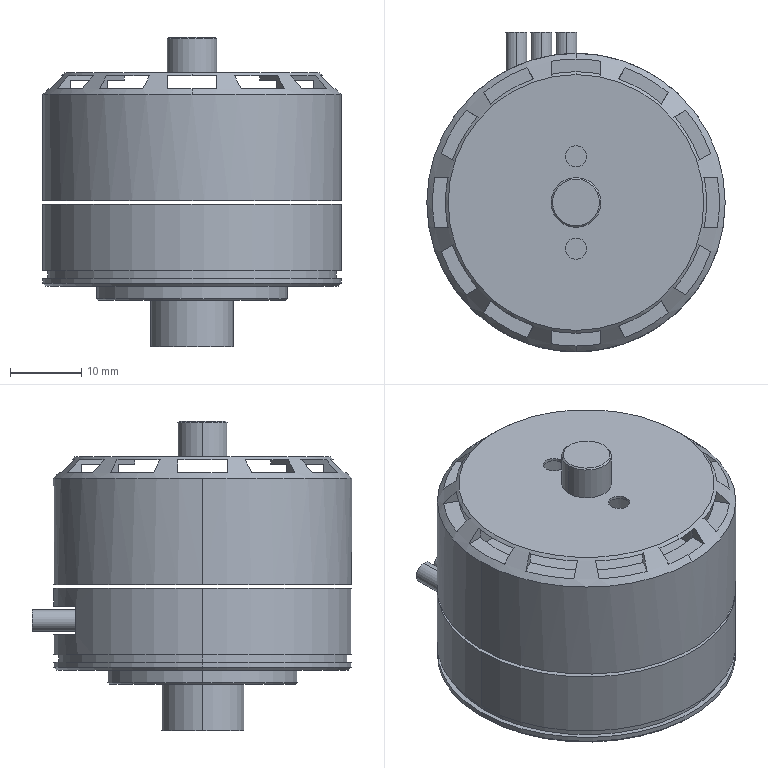Part | SolidWorks | features BaseBody 2 | 2 solids | 111 faces | box 42 x 45 x 43.5 mm | volume 22402 mm3 | plane 69 | cylinder 34 | cone 8 | commonest cylinder face diameters 3 x18 42 x6 7 x2 11.6 x2 26.8 x2 36 x2